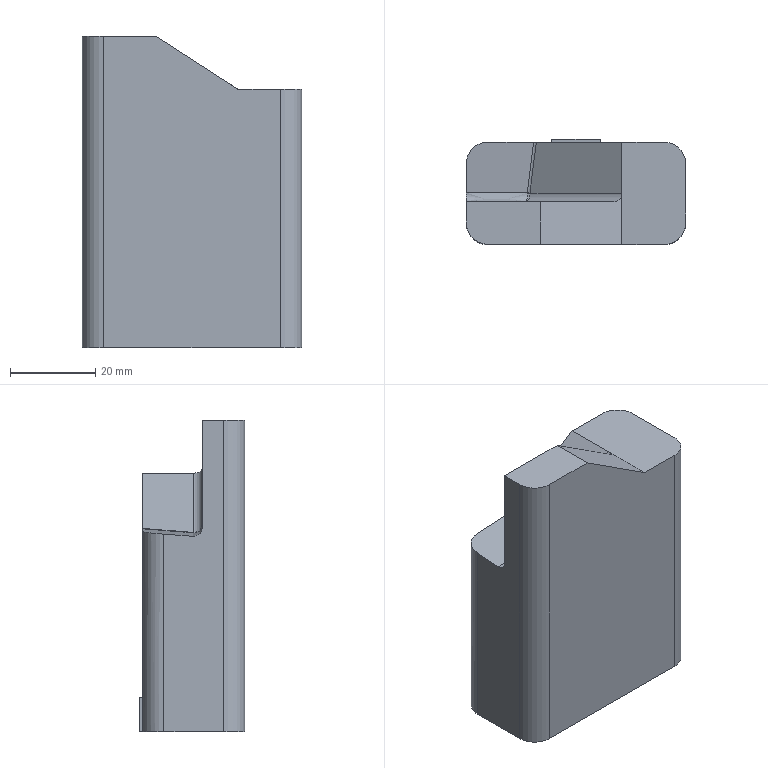Part | STEP file | gslz 2016.10.28-13_id1366_x_t | 1 solid | 24 faces | box 51.5 x 24.8 x 73 mm | volume 72067 mm3 | plane 14 | cylinder 5 | spline 5 | commonest cylinder face diameters 10 x4 4 x1